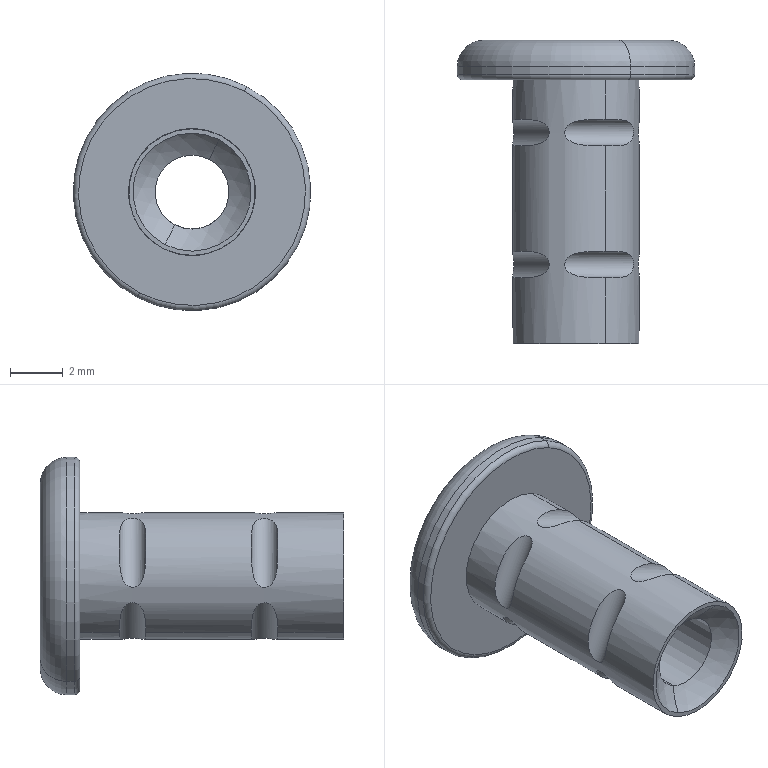Part | SolidWorks | features BaseBody 1 | 1 solid | 43 faces | box 9 x 11.503 x 9 mm | volume 190.37 mm3 | plane 23 | cylinder 14 | torus 4 | sphere 2 | commonest cylinder face diameters 1 x8 2.8 x2 4.8 x2 9 x2